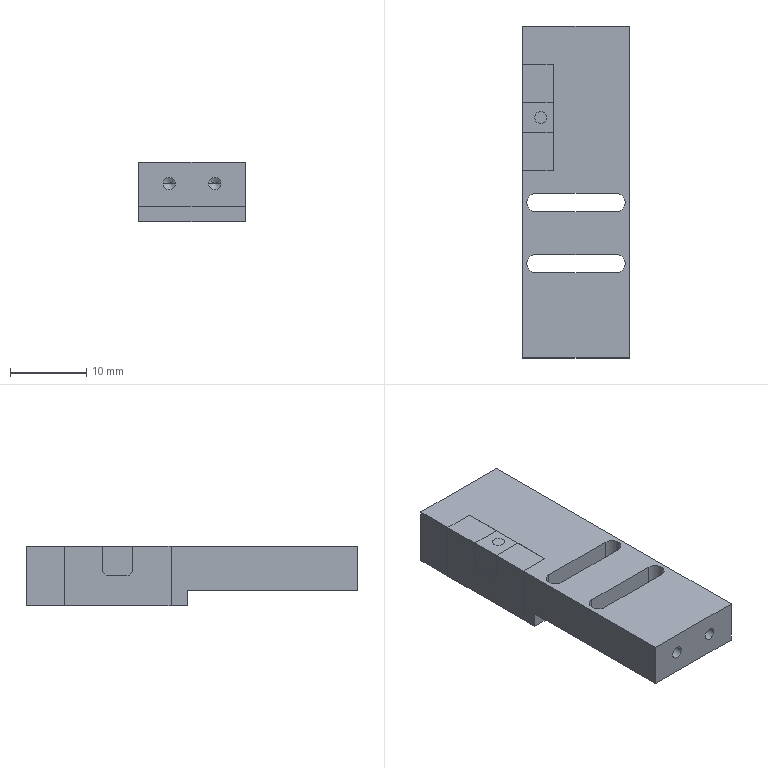NC program | NX | posted with a generic post | part box 14 x 43.5 x 7.8 mm
Whole program:
N10 G17 G21 G94 G90
(FLOOR_WALL , TOOL : D10JING)
N12 T09 M6
N14 G54
N16 G17 G0 G90 X31.75 Y-8.997 B0. C0. S9500 M3
N18 G43 Z30. H9
N20 Z3.
N22 G94 G1 Z0. F1250.
N24 X28.75
N26 X-28.75
N28 Y-4.331
N30 X28.75
N32 Y0.334
N34 X-28.75
N36 Y5.
N38 X28.75
N40 X31.75
N42 Z3.
N44 G0 Z30.
N46 M5
(DRILLING_COPY_1 , TOOL : D6A45)
N48 T07 M6
N50 G54
N52 G17 G0 G90 X-9.75 Y4.6 B0. C0. S5000 M3
N54 G43 Z30. H7
N56 G94 G81 G98 Z-1. F250. R3.
N58 X5.39 Y3.5
N60 G80
N62 G0 X5.39 Y3.5 Z30.
N64 M5
(DRILLING_COPY_COPY_COPY , TOOL : 1.6ZT)
N66 T14 M6
N68 G54
N70 G17 G0 G90 X-9.75 Y4.6 B0. C0. S2000 M3
N72 G43 Z30. H14
N74 G94 G83 G98 Z-9.781 F150. Q2. R3.
N76 X5.39 Y3.5 Z-6.481
N78 G80
N80 G0 X5.39 Y3.5 Z30.
N82 M5
(ZLEVEL_PROFILE , TOOL : D10)
N84 T10 M6
N86 G54
N88 G17 G0 G90 X14.075 Y12.1 B0. C0. S9500 M3
N90 G43 Z30. H10
N92 Z1.5
N94 G94 G1 X22.304 Z1.069 F1000.
N96 X23.648 Y11.766 Z0.996
N98 X24.854 Y11.084 Z0.924
N100 X25.834 Y10.104 Z0.851
N102 X26.516 Y8.898 Z0.778
N104 X26.85 Y7.554 Z0.706
N106 Y-7.554 Z-0.086
N108 X26.516 Y-8.898 Z-0.159
N110 X25.834 Y-10.104 Z-0.231
N112 X24.854 Y-11.084 Z-0.304
N114 X23.648 Y-11.766 Z-0.376
N116 X22.304 Y-12.1 Z-0.449
N118 X21.75 Z-0.478
N120 X-21.75 F2500.
N122 G2 X-26.85 Y-7. R5.1
N124 G1 Y7.
N126 G2 X-21.75 Y12.1 R5.1
N128 G1 X21.75
N130 G2 X26.85 Y7. R5.1
N132 G1 Y-7.
N134 G2 X21.75 Y-12.1 R5.1
N136 G1 X-5.642 Z-0.956
N138 X-21.75
N140 G2 X-26.85 Y-7. R5.1
N142 G1 Y7.
N144 G2 X-21.75 Y12.1 R5.1
N146 G1 X21.75
N148 G2 X26.85 Y7. R5.1
N150 G1 Y-7.
N152 G2 X21.75 Y-12.1 R5.1
N154 G1 X-5.642 Z-1.434
N156 X-21.75
N158 G2 X-26.85 Y-7. R5.1
N160 G1 Y7.
N162 G2 X-21.75 Y12.1 R5.1
N164 G1 X21.75
N166 G2 X26.85 Y7. R5.1
N168 G1 Y-7.
N170 G2 X21.75 Y-12.1 R5.1
N172 G1 X-5.642 Z-1.913
N174 X-21.75
N176 G2 X-26.85 Y-7. R5.1
N178 G1 Y7.
N180 G2 X-21.75 Y12.1 R5.1
N182 G1 X21.75
N184 G2 X26.85 Y7. R5.1
N186 G1 Y-7.
N188 G2 X21.75 Y-12.1 R5.1
N190 G1 X-5.642 Z-2.391
N192 X-21.75
N194 G2 X-26.85 Y-7. R5.1
N196 G1 Y7.
N198 G2 X-21.75 Y12.1 R5.1
N200 G1 X21.75
N202 G2 X26.85 Y7. R5.1
N204 G1 Y-7.
N206 G2 X21.75 Y-12.1 R5.1
N208 G1 X-5.642 Z-2.869
N210 X-21.75
N212 G2 X-26.85 Y-7. R5.1
N214 G1 Y7.
N216 G2 X-21.75 Y12.1 R5.1
N218 G1 X21.75
N220 G2 X26.85 Y7. R5.1
N222 G1 Y-7.
N224 G2 X21.75 Y-12.1 R5.1
N226 G1 X-5.642 Z-3.347
N228 X-21.75
N230 G2 X-26.85 Y-7. R5.1
N232 G1 Y7.
N234 G2 X-21.75 Y12.1 R5.1
N236 G1 X21.75
N238 G2 X26.85 Y7. R5.1
N240 G1 Y-7.
N242 G2 X21.75 Y-12.1 R5.1
N244 G1 X-5.642 Z-3.825
N246 X-21.75
N248 G2 X-26.85 Y-7. R5.1
N250 G1 Y7.
N252 G2 X-21.75 Y12.1 R5.1
N254 G1 X21.75
N256 G2 X26.85 Y7. R5.1
N258 G1 Y-7.
N260 G2 X21.75 Y-12.1 R5.1
N262 G1 X-5.642 Z-4.303
N264 X-21.75
N266 G2 X-26.85 Y-7. R5.1
N268 G1 Y7.
N270 G2 X-21.75 Y12.1 R5.1
N272 G1 X21.75
N274 G2 X26.85 Y7. R5.1
N276 G1 Y-7.
N278 G2 X21.75 Y-12.1 R5.1
N280 G1 X-5.642 Z-4.781
N282 X-21.75
N284 G2 X-26.85 Y-7. R5.1
N286 G1 Y7.
N288 G2 X-21.75 Y12.1 R5.1
N290 G1 X21.75
N292 G2 X26.85 Y7. R5.1
N294 G1 Y-7.
N296 G2 X21.75 Y-12.1 R5.1
N298 G1 X-5.642 Z-5.259
N300 X-21.75
N302 G2 X-26.85 Y-7. R5.1
N304 G1 Y7.
N306 G2 X-21.75 Y12.1 R5.1
N308 G1 X21.75
N310 G2 X26.85 Y7. R5.1
N312 G1 Y-7.
N314 G2 X21.75 Y-12.1 R5.1
N316 G1 X-5.642 Z-5.738
N318 X-21.75
N320 G2 X-26.85 Y-7. R5.1
N322 G1 Y7.
N324 G2 X-21.75 Y12.1 R5.1
N326 G1 X21.75
N328 G2 X26.85 Y7. R5.1
N330 G1 Y-7.
N332 G2 X21.75 Y-12.1 R5.1
N334 G1 X-5.642 Z-6.216
N336 X-21.75
N338 G2 X-26.85 Y-7. R5.1
N340 G1 Y7.
N342 G2 X-21.75 Y12.1 R5.1
N344 G1 X21.75
N346 G2 X26.85 Y7. R5.1
N348 G1 Y-7.
N350 G2 X21.75 Y-12.1 R5.1
N352 G1 X-5.642 Z-6.694
N354 X-21.75
N356 G2 X-26.85 Y-7. R5.1
N358 G1 Y7.
N360 G2 X-21.75 Y12.1 R5.1
N362 G1 X21.75
N364 G2 X26.85 Y7. R5.1
N366 G1 Y-7.
N368 G2 X21.75 Y-12.1 R5.1
N370 G1 X-5.642 Z-7.172
N372 X-21.75
N374 G2 X-26.85 Y-7. R5.1
N376 G1 Y7.
N378 G2 X-21.75 Y12.1 R5.1
N380 G1 X21.75
N382 G2 X26.85 Y7. R5.1
N384 G1 Y-7.
N386 G2 X21.75 Y-12.1 R5.1
N388 G1 X-5.642 Z-7.65
N390 X-21.75
N392 G2 X-26.85 Y-7. R5.1
N394 G1 Y7.
N396 G2 X-21.75 Y12.1 R5.1
N398 G1 X21.75
N400 G2 X26.85 Y7. R5.1
N402 G1 Y-7.
N404 G2 X21.75 Y-12.1 R5.1
N406 G1 X-5.642
N408 Z-6.15
N410 G0 Z30.
N412 M5
(FLOOR_WALL_1 , TOOL : D6)
N414 T06 M6
N416 G54
N418 G17 G0 G90 X12.12 Y12. B0. C0. S9500 M3
N420 G43 Z30. H6
N422 Z0.525
N424 G94 G1 Z-0.475 F1000.
N426 Y7.
N428 X21.75 F2500.
N430 Y-7.
N432 X2.49
N434 Y7.
N436 X12.12
N438 Y4.
N440 X18.75
N442 Y-4.
N444 X5.49
N446 Y4.
N448 X12.12
N450 Y1.
N452 X15.75
N454 Y-1.
N456 X8.49
N458 Y1.
N460 X12.12
N462 Y2.
N464 Z0.525
N466 G0 Y12. Z0.05
N468 G1 Z-0.95 F1000.
N470 Y7.
N472 X21.75 F2500.
N474 Y-7.
N476 X2.49
N478 Y7.
N480 X12.12
N482 Y4.
N484 X18.75
N486 Y-4.
N488 X5.49
N490 Y4.
N492 X12.12
N494 Y1.
N496 X15.75
N498 Y-1.
N500 X8.49
N502 Y1.
N504 X12.12
N506 Y2.
N508 Z0.05
N510 G0 Y12. Z-0.425
N512 G1 Z-1.425 F1000.
N514 Y7.
N516 X21.75 F2500.
N518 Y-7.
N520 X2.49
N522 Y7.
N524 X12.12
N526 Y4.
N528 X18.75
N530 Y-4.
N532 X5.49
N534 Y4.
N536 X12.12
N538 Y1.
N540 X15.75
N542 Y-1.
N544 X8.49
N546 Y1.
N548 X12.12
N550 Y2.
N552 Z-0.425
N554 G0 Y12. Z-0.9
N556 G1 Z-1.9 F1000.
N558 Y7.
N560 X21.75 F2500.
N562 Y-7.
N564 X2.49
N566 Y7.
N568 X12.12
N570 Y4.
N572 X18.75
N574 Y-4.
N576 X5.49
N578 Y4.
N580 X12.12
N582 Y1.
N584 X15.75
N586 Y-1.
N588 X8.49
N590 Y1.
N592 X12.12
N594 Y2.
N596 Z-0.9
N598 G0 Z30.
(FLOOR_WALL_1_COPY , TOOL : D6)
N600 X21.747 Y12.
N602 Z-1.
N604 G1 Z-2. F1000.
N606 Y10.
N608 Y-10. F1200.
N610 X19.025
N612 Y10.
N614 X16.302
N616 Y-10.
N618 X13.58
N620 Y10.
N622 X10.857
N624 Y-10.
N626 X8.135
N628 Y10.
N630 X5.412
N632 Y-10.
N634 X2.69
N636 Y10.
N638 Y12.
N640 Z-1.
N642 G0 X2.39
N644 G1 Z-2. F1000.
N646 Y10.
N648 Y-10. F1200.
N650 Y-12.
N652 Z-1.
N654 G0 Z30.
N656 M5
(ZLEVEL_PROFILE_COPY_COPY_COPY , TOOL : D1.5)
N658 T13 M6
N660 G54
N662 G17 G0 G90 X1.84 Y0.019 B0. C0. S9500 M3
N664 G43 Z30. H13
N666 Z-0.5
N668 G94 G1 Y5.345 Z-0.779 F1000.
N670 X1.754 Y5.531 Z-0.79
N672 X1.597 Y5.661 Z-0.801
N674 X1.398 Y5.71 Z-0.811
N676 X1.211 Y5.674 Z-0.821
N678 X1.035 Y5.543 Z-0.833
N680 X0.94 Y5.345 Z-0.844
N682 Y-5.345 Z-1.405
N684 X1.026 Y-5.531 Z-1.415
N686 X1.183 Y-5.661 Z-1.426
N688 X1.382 Y-5.71 Z-1.437
N690 X1.569 Y-5.674 Z-1.447
N692 X1.745 Y-5.543 Z-1.458
N694 X1.84 Y-5.345 Z-1.47
N696 Y5.345 Z-2.03
N698 X1.754 Y5.531 Z-2.041
N700 X1.597 Y5.661 Z-2.051
N702 X1.398 Y5.71 Z-2.062
N704 X1.211 Y5.674 Z-2.072
N706 X1.035 Y5.543 Z-2.084
N708 X0.94 Y5.345 Z-2.095
N710 Y5.25 Z-2.1
N712 Y-5.25
N714 G3 X1.39 Y-5.7 R0.45
N716 X1.84 Y-5.25 R0.45
N718 G1 Y5.25
N720 G3 X1.39 Y5.7 R0.45
N722 X0.94 Y5.25 R0.45
N724 G1 Y-0.479 Z-2.2
N726 Y-5.25
N728 G3 X1.39 Y-5.7 R0.45
N730 X1.84 Y-5.25 R0.45
N732 G1 Y5.25
N734 G3 X1.39 Y5.7 R0.45
N736 X0.94 Y5.25 R0.45
N738 G1 Y-0.479 Z-2.3
N740 Y-5.25
N742 G3 X1.39 Y-5.7 R0.45
N744 X1.84 Y-5.25 R0.45
N746 G1 Y5.25
N748 G3 X1.39 Y5.7 R0.45
N750 X0.94 Y5.25 R0.45
N752 G1 Y-0.479 Z-2.4
N754 Y-5.25
N756 G3 X1.39 Y-5.7 R0.45
N758 X1.84 Y-5.25 R0.45
N760 G1 Y5.25
N762 G3 X1.39 Y5.7 R0.45
N764 X0.94 Y5.25 R0.45
N766 G1 Y-0.479 Z-2.5
N768 Y-5.25
N770 G3 X1.39 Y-5.7 R0.45
N772 X1.84 Y-5.25 R0.45
N774 G1 Y5.25
N776 G3 X1.39 Y5.7 R0.45
N778 X0.94 Y5.25 R0.45
N780 G1 Y-0.479 Z-2.6
N782 Y-5.25
N784 G3 X1.39 Y-5.7 R0.45
N786 X1.84 Y-5.25 R0.45
N788 G1 Y5.25
N790 G3 X1.39 Y5.7 R0.45
N792 X0.94 Y5.25 R0.45
N794 G1 Y-0.479 Z-2.7
N796 Y-5.25
N798 G3 X1.39 Y-5.7 R0.45
N800 X1.84 Y-5.25 R0.45
N802 G1 Y5.25
N804 G3 X1.39 Y5.7 R0.45
N806 X0.94 Y5.25 R0.45
N808 G1 Y-0.479 Z-2.8
N810 Y-5.25
N812 G3 X1.39 Y-5.7 R0.45
N814 X1.84 Y-5.25 R0.45
N816 G1 Y5.25
N818 G3 X1.39 Y5.7 R0.45
N820 X0.94 Y5.25 R0.45
N822 G1 Y-0.479 Z-2.9
N824 Y-5.25
N826 G3 X1.39 Y-5.7 R0.45
N828 X1.84 Y-5.25 R0.45
N830 G1 Y5.25
N832 G3 X1.39 Y5.7 R0.45
N834 X0.94 Y5.25 R0.45
N836 G1 Y-0.479 Z-3.
N838 Y-5.25
N840 G3 X1.39 Y-5.7 R0.45
N842 X1.84 Y-5.25 R0.45
N844 G1 Y5.25
N846 G3 X1.39 Y5.7 R0.45
N848 X0.94 Y5.25 R0.45
N850 G1 Y-0.479 Z-3.1
N852 Y-5.25
N854 G3 X1.39 Y-5.7 R0.45
N856 X1.84 Y-5.25 R0.45
N858 G1 Y5.25
N860 G3 X1.39 Y5.7 R0.45
N862 X0.94 Y5.25 R0.45
N864 G1 Y-0.479 Z-3.2
N866 Y-5.25
N868 G3 X1.39 Y-5.7 R0.45
N870 X1.84 Y-5.25 R0.45
N872 G1 Y5.25
N874 G3 X1.39 Y5.7 R0.45
N876 X0.94 Y5.25 R0.45
N878 G1 Y-0.479 Z-3.3
N880 Y-5.25
N882 G3 X1.39 Y-5.7 R0.45
N884 X1.84 Y-5.25 R0.45
N886 G1 Y5.25
N888 G3 X1.39 Y5.7 R0.45
N890 X0.94 Y5.25 R0.45
N892 G1 Y-0.479 Z-3.4
N894 Y-5.25
N896 G3 X1.39 Y-5.7 R0.45
N898 X1.84 Y-5.25 R0.45
N900 G1 Y5.25
N902 G3 X1.39 Y5.7 R0.45
N904 X0.94 Y5.25 R0.45
N906 G1 Y-0.479 Z-3.5
N908 Y-5.25
N910 G3 X1.39 Y-5.7 R0.45
N912 X1.84 Y-5.25 R0.45
N914 G1 Y5.25
N916 G3 X1.39 Y5.7 R0.45
N918 X0.94 Y5.25 R0.45
N920 G1 Y-0.479 Z-3.6
N922 Y-5.25
N924 G3 X1.39 Y-5.7 R0.45
N926 X1.84 Y-5.25 R0.45
N928 G1 Y5.25
N930 G3 X1.39 Y5.7 R0.45
N932 X0.94 Y5.25 R0.45
N934 G1 Y-0.479 Z-3.7
N936 Y-5.25
N938 G3 X1.39 Y-5.7 R0.45
N940 X1.84 Y-5.25 R0.45
N942 G1 Y5.25
N944 G3 X1.39 Y5.7 R0.45
N946 X0.94 Y5.25 R0.45
N948 G1 Y-0.479 Z-3.8
N950 Y-5.25
N952 G3 X1.39 Y-5.7 R0.45
N954 X1.84 Y-5.25 R0.45
N956 G1 Y5.25
N958 G3 X1.39 Y5.7 R0.45
N960 X0.94 Y5.25 R0.45
N962 G1 Y-0.479 Z-3.9
N964 Y-5.25
N966 G3 X1.39 Y-5.7 R0.45
N968 X1.84 Y-5.25 R0.45
N970 G1 Y5.25
N972 G3 X1.39 Y5.7 R0.45
N974 X0.94 Y5.25 R0.45
N976 G1 Y-0.479 Z-4.
N978 Y-5.25
N980 G3 X1.39 Y-5.7 R0.45
N982 X1.84 Y-5.25 R0.45
N984 G1 Y5.25
N986 G3 X1.39 Y5.7 R0.45
N988 X0.94 Y5.25 R0.45
N990 G1 Y-0.479 Z-4.1
N992 Y-5.25
N994 G3 X1.39 Y-5.7 R0.45
N996 X1.84 Y-5.25 R0.45
N998 G1 Y5.25
N1000 G3 X1.39 Y5.7 R0.45
N1002 X0.94 Y5.25 R0.45
N1004 G1 Y-0.479 Z-4.2
N1006 Y-5.25
N1008 G3 X1.39 Y-5.7 R0.45
N1010 X1.84 Y-5.25 R0.45
N1012 G1 Y5.25
N1014 G3 X1.39 Y5.7 R0.45
N1016 X0.94 Y5.25 R0.45
N1018 G1 Y-0.479 Z-4.3
N1020 Y-5.25
N1022 G3 X1.39 Y-5.7 R0.45
N1024 X1.84 Y-5.25 R0.45
N1026 G1 Y5.25
N1028 G3 X1.39 Y5.7 R0.45
N1030 X0.94 Y5.25 R0.45
N1032 G1 Y-0.479 Z-4.4
N1034 Y-5.25
N1036 G3 X1.39 Y-5.7 R0.45
N1038 X1.84 Y-5.25 R0.45
N1040 G1 Y5.25
N1042 G3 X1.39 Y5.7 R0.45
N1044 X0.94 Y5.25 R0.45
N1046 G1 Y-0.479 Z-4.5
N1048 Y-5.25
N1050 G3 X1.39 Y-5.7 R0.45
N1052 X1.84 Y-5.25 R0.45
N1054 G1 Y5.25
N1056 G3 X1.39 Y5.7 R0.45
N1058 X0.94 Y5.25 R0.45
N1060 G1 Y-0.479 Z-4.6
N1062 Y-5.25
N1064 G3 X1.39 Y-5.7 R0.45
N1066 X1.84 Y-5.25 R0.45
N1068 G1 Y5.25
N1070 G3 X1.39 Y5.7 R0.45
N1072 X0.94 Y5.25 R0.45
N1074 G1 Y-0.479 Z-4.7
N1076 Y-5.25
N1078 G3 X1.39 Y-5.7 R0.45
N1080 X1.84 Y-5.25 R0.45
N1082 G1 Y5.25
N1084 G3 X1.39 Y5.7 R0.45
N1086 X0.94 Y5.25 R0.45
N1088 G1 Y-0.479 Z-4.8
N1090 Y-5.25
N1092 G3 X1.39 Y-5.7 R0.45
N1094 X1.84 Y-5.25 R0.45
N1096 G1 Y5.25
N1098 G3 X1.39 Y5.7 R0.45
N1100 X0.94 Y5.25 R0.45
N1102 G1 Y-0.479 Z-4.9
N1104 Y-5.25
N1106 G3 X1.39 Y-5.7 R0.45
N1108 X1.84 Y-5.25 R0.45
N1110 G1 Y5.25
N1112 G3 X1.39 Y5.7 R0.45
N1114 X0.94 Y5.25 R0.45
N1116 G1 Y-0.479 Z-5.
N1118 Y-5.25
N1120 G3 X1.39 Y-5.7 R0.45
N1122 X1.84 Y-5.25 R0.45
N1124 G1 Y5.25
N1126 G3 X1.39 Y5.7 R0.45
N1128 X0.94 Y5.25 R0.45
N1130 G1 Y-0.479 Z-5.1
N1132 Y-5.25
N1134 G3 X1.39 Y-5.7 R0.45
N1136 X1.84 Y-5.25 R0.45
N1138 G1 Y5.25
N1140 G3 X1.39 Y5.7 R0.45
N1142 X0.94 Y5.25 R0.45
N1144 G1 Y-0.479 Z-5.2
N1146 Y-5.25
N1148 G3 X1.39 Y-5.7 R0.45
N1150 X1.84 Y-5.25 R0.45
N1152 G1 Y5.25
N1154 G3 X1.39 Y5.7 R0.45
N1156 X0.94 Y5.25 R0.45
N1158 G1 Y-0.479 Z-5.3
N1160 Y-5.25
N1162 G3 X1.39 Y-5.7 R0.45
N1164 X1.84 Y-5.25 R0.45
N1166 G1 Y5.25
N1168 G3 X1.39 Y5.7 R0.45
N1170 X0.94 Y5.25 R0.45
N1172 G1 Y-0.479 Z-5.4
N1174 Y-5.25
N1176 G3 X1.39 Y-5.7 R0.45
N1178 X1.84 Y-5.25 R0.45
N1180 G1 Y5.25
N1182 G3 X1.39 Y5.7 R0.45
N1184 X0.94 Y5.25 R0.45
N1186 G1 Y-0.479 Z-5.5
N1188 Y-5.25
N1190 G3 X1.39 Y-5.7 R0.45
N1192 X1.84 Y-5.25 R0.45
N1194 G1 Y5.25
N1196 G3 X1.39 Y5.7 R0.45
N1198 X0.94 Y5.25 R0.45
N1200 G1 Y-0.479 Z-5.6
N1202 Y-5.25
N1204 G3 X1.39 Y-5.7 R0.45
N1206 X1.84 Y-5.25 R0.45
N1208 G1 Y5.25
N1210 G3 X1.39 Y5.7 R0.45
N1212 X0.94 Y5.25 R0.45
N1214 G1 Y-0.479 Z-5.7
N1216 Y-5.25
N1218 G3 X1.39 Y-5.7 R0.45
N1220 X1.84 Y-5.25 R0.45
N1222 G1 Y5.25
N1224 G3 X1.39 Y5.7 R0.45
N1226 X0.94 Y5.25 R0.45
N1228 G1 Y-0.479 Z-5.8
N1230 Y-5.25
N1232 G3 X1.39 Y-5.7 R0.45
N1234 X1.84 Y-5.25 R0.45
N1236 G1 Y5.25
N1238 G3 X1.39 Y5.7 R0.45
N1240 X0.94 Y5.25 R0.45
N1242 G1 Y-0.479 Z-5.9
N1244 Y-5.25
N1246 G3 X1.39 Y-5.7 R0.45
N1248 X1.84 Y-5.25 R0.45
N1250 G1 Y5.25
N1252 G3 X1.39 Y5.7 R0.45
N1254 X0.94 Y5.25 R0.45
N1256 G1 Y-0.479 Z-6.
N1258 Y-5.25
N1260 G3 X1.39 Y-5.7 R0.45
N1262 X1.84 Y-5.25 R0.45
N1264 G1 Y5.25
N1266 G3 X1.39 Y5.7 R0.45
N1268 X0.94 Y5.25 R0.45
N1270 G1 Y-0.479 Z-6.1
N1272 Y-5.25
N1274 G3 X1.39 Y-5.7 R0.45
N1276 X1.84 Y-5.25 R0.45
N1278 G1 Y5.25
N1280 G3 X1.39 Y5.7 R0.45
N1282 X0.94 Y5.25 R0.45
N1284 G1 Y-0.479 Z-6.2
N1286 Y-5.25
N1288 G3 X1.39 Y-5.7 R0.45
N1290 X1.84 Y-5.25 R0.45
N1292 G1 Y5.25
N1294 G3 X1.39 Y5.7 R0.45
N1296 X0.94 Y5.25 R0.45
N1298 G1 Y-0.479 Z-6.3
N1300 Y-5.25
N1302 G3 X1.39 Y-5.7 R0.45
N1304 X1.84 Y-5.25 R0.45
N1306 G1 Y5.25
N1308 G3 X1.39 Y5.7 R0.45
N1310 X0.94 Y5.25 R0.45
N1312 G1 Y-0.479 Z-6.4
N1314 Y-5.25
N1316 G3 X1.39 Y-5.7 R0.45
N1318 X1.84 Y-5.25 R0.45
N1320 G1 Y5.25
N1322 G3 X1.39 Y5.7 R0.45
N1324 X0.94 Y5.25 R0.45
N1326 G1 Y-0.479 Z-6.5
N1328 Y-5.25
N1330 G3 X1.39 Y-5.7 R0.45
N1332 X1.84 Y-5.25 R0.45
N1334 G1 Y5.25
N1336 G3 X1.39 Y5.7 R0.45
N1338 X0.94 Y5.25 R0.45
N1340 G1 Y-0.479 Z-6.6
N1342 Y-5.25
N1344 G3 X1.39 Y-5.7 R0.45
N1346 X1.84 Y-5.25 R0.45
N1348 G1 Y5.25
N1350 G3 X1.39 Y5.7 R0.45
N1352 X0.94 Y5.25 R0.45
N1354 G1 Y-0.479 Z-6.7
N1356 Y-5.25
N1358 G3 X1.39 Y-5.7 R0.45
N1360 X1.84 Y-5.25 R0.45
N1362 G1 Y5.25
N1364 G3 X1.39 Y5.7 R0.45
N1366 X0.94 Y5.25 R0.45
N1368 G1 Y-0.479 Z-6.8
N1370 Y-5.25
N1372 G3 X1.39 Y-5.7 R0.45
N1374 X1.84 Y-5.25 R0.45
N1376 G1 Y5.25
N1378 G3 X1.39 Y5.7 R0.45
N1380 X0.94 Y5.25 R0.45
N1382 G1 Y-0.479 Z-6.9
N1384 Y-5.25
N1386 G3 X1.39 Y-5.7 R0.45
N1388 X1.84 Y-5.25 R0.45
N1390 G1 Y5.25
N1392 G3 X1.39 Y5.7 R0.45
N1394 X0.94 Y5.25 R0.45
N1396 G1 Y-0.479 Z-7.
N1398 Y-5.25
N1400 G3 X1.39 Y-5.7 R0.45
N1402 X1.84 Y-5.25 R0.45
N1404 G1 Y5.25
N1406 G3 X1.39 Y5.7 R0.45
N1408 X0.94 Y5.25 R0.45
N1410 G1 Y-0.479 Z-7.1
N1412 Y-5.25
N1414 G3 X1.39 Y-5.7 R0.45
N1416 X1.84 Y-5.25 R0.45
N1418 G1 Y5.25
N1420 G3 X1.39 Y5.7 R0.45
N1422 X0.94 Y5.25 R0.45
N1424 G1 Y-0.479 Z-7.2
N1426 Y-5.25
N1428 G3 X1.39 Y-5.7 R0.45
N1430 X1.84 Y-5.25 R0.45
N1432 G1 Y5.25
N1434 G3 X1.39 Y5.7 R0.45
N1436 X0.94 Y5.25 R0.45
N1438 G1 Y-0.479 Z-7.3
N1440 Y-5.25
N1442 G3 X1.39 Y-5.7 R0.45
N1444 X1.84 Y-5.25 R0.45
N1446 G1 Y5.25
N1448 G3 X1.39 Y5.7 R0.45
N1450 X0.94 Y5.25 R0.45
N1452 G1 Y-0.479 Z-7.4
N1454 Y-5.25
N1456 G3 X1.39 Y-5.7 R0.45
N1458 X1.84 Y-5.25 R0.45
N1460 G1 Y5.25
N1462 G3 X1.39 Y5.7 R0.45
N1464 X0.94 Y5.25 R0.45
N1466 G1 Y-0.479 Z-7.5
N1468 Y-5.25
N1470 G3 X1.39 Y-5.7 R0.45
N1472 X1.84 Y-5.25 R0.45
N1474 G1 Y5.25
N1476 G3 X1.39 Y5.7 R0.45
N1478 X0.94 Y5.25 R0.45
N1480 G1 Y-0.479 Z-7.6
N1482 Y-5.25
N1484 G3 X1.39 Y-5.7 R0.45
N1486 X1.84 Y-5.25 R0.45
N1488 G1 Y5.25
N1490 G3 X1.39 Y5.7 R0.45
N1492 X0.94 Y5.25 R0.45
N1494 G1 Y-0.479 Z-7.7
N1496 Y-5.25
N1498 G3 X1.39 Y-5.7 R0.45
N1500 X1.84 Y-5.25 R0.45
N1502 G1 Y5.25
N1504 G3 X1.39 Y5.7 R0.45
N1506 X0.94 Y5.25 R0.45
N1508 G1 Y-0.479 Z-7.8
N1510 Y-5.25
N1512 G3 X1.39 Y-5.7 R0.45
N1514 X1.84 Y-5.25 R0.45
N1516 G1 Y5.25
N1518 G3 X1.39 Y5.7 R0.45
N1520 X0.94 Y5.25 R0.45
N1522 G1 Y-0.479
N1524 Z-6.3
N1526 G0 Z30.
N1528 X9.84 Y0.019
N1530 Z-0.5
N1532 G1 Y5.345 Z-0.779
N1534 X9.754 Y5.531 Z-0.79
N1536 X9.597 Y5.661 Z-0.801
N1538 X9.398 Y5.71 Z-0.811
N1540 X9.211 Y5.674 Z-0.821
N1542 X9.035 Y5.543 Z-0.833
N1544 X8.94 Y5.345 Z-0.844
N1546 Y-5.345 Z-1.405
N1548 X9.026 Y-5.531 Z-1.415
N1550 X9.183 Y-5.661 Z-1.426
N1552 X9.382 Y-5.71 Z-1.437
N1554 X9.569 Y-5.674 Z-1.447
N1556 X9.745 Y-5.543 Z-1.458
N1558 X9.84 Y-5.345 Z-1.47
N1560 Y5.345 Z-2.03
N1562 X9.754 Y5.531 Z-2.041
N1564 X9.597 Y5.661 Z-2.051
N1566 X9.398 Y5.71 Z-2.062
N1568 X9.211 Y5.674 Z-2.072
N1570 X9.035 Y5.543 Z-2.084
N1572 X8.94 Y5.345 Z-2.095
N1574 Y5.25 Z-2.1
N1576 Y-5.25
N1578 G3 X9.39 Y-5.7 R0.45
N1580 X9.84 Y-5.25 R0.45
N1582 G1 Y5.25
N1584 G3 X9.39 Y5.7 R0.45
N1586 X8.94 Y5.25 R0.45
N1588 G1 Y-0.479 Z-2.2
N1590 Y-5.25
N1592 G3 X9.39 Y-5.7 R0.45
N1594 X9.84 Y-5.25 R0.45
N1596 G1 Y5.25
N1598 G3 X9.39 Y5.7 R0.45
N1600 X8.94 Y5.25 R0.45
N1602 G1 Y-0.479 Z-2.3
N1604 Y-5.25
N1606 G3 X9.39 Y-5.7 R0.45
N1608 X9.84 Y-5.25 R0.45
N1610 G1 Y5.25
N1612 G3 X9.39 Y5.7 R0.45
N1614 X8.94 Y5.25 R0.45
N1616 G1 Y-0.479 Z-2.4
N1618 Y-5.25
N1620 G3 X9.39 Y-5.7 R0.45
N1622 X9.84 Y-5.25 R0.45
N1624 G1 Y5.25
N1626 G3 X9.39 Y5.7 R0.45
N1628 X8.94 Y5.25 R0.45
N1630 G1 Y-0.479 Z-2.5
N1632 Y-5.25
N1634 G3 X9.39 Y-5.7 R0.45
N1636 X9.84 Y-5.25 R0.45
N1638 G1 Y5.25
N1640 G3 X9.39 Y5.7 R0.45
N1642 X8.94 Y5.25 R0.45
N1644 G1 Y-0.479 Z-2.6
N1646 Y-5.25
N1648 G3 X9.39 Y-5.7 R0.45
N1650 X9.84 Y-5.25 R0.45
N1652 G1 Y5.25
N1654 G3 X9.39 Y5.7 R0.45
N1656 X8.94 Y5.25 R0.45
N1658 G1 Y-0.479 Z-2.7
N1660 Y-5.25
N1662 G3 X9.39 Y-5.7 R0.45
N1664 X9.84 Y-5.25 R0.45
N1666 G1 Y5.25
N1668 G3 X9.39 Y5.7 R0.45
N1670 X8.94 Y5.25 R0.45
N1672 G1 Y-0.479 Z-2.8
N1674 Y-5.25
N1676 G3 X9.39 Y-5.7 R0.45
N1678 X9.84 Y-5.25 R0.45
N1680 G1 Y5.25
N1682 G3 X9.39 Y5.7 R0.45
N1684 X8.94 Y5.25 R0.45
N1686 G1 Y-0.479 Z-2.9
N1688 Y-5.25
N1690 G3 X9.39 Y-5.7 R0.45
N1692 X9.84 Y-5.25 R0.45
N1694 G1 Y5.25
N1696 G3 X9.39 Y5.7 R0.45
N1698 X8.94 Y5.25 R0.45
N1700 G1 Y-0.479 Z-3.
N1702 Y-5.25
N1704 G3 X9.39 Y-5.7 R0.45
N1706 X9.84 Y-5.25 R0.45
N1708 G1 Y5.25
N1710 G3 X9.39 Y5.7 R0.45
N1712 X8.94 Y5.25 R0.45
N1714 G1 Y-0.479 Z-3.1
N1716 Y-5.25
N1718 G3 X9.39 Y-5.7 R0.45
N1720 X9.84 Y-5.25 R0.45
N1722 G1 Y5.25
N1724 G3 X9.39 Y5.7 R0.45
N1726 X8.94 Y5.25 R0.45
N1728 G1 Y-0.479 Z-3.2
N1730 Y-5.25
N1732 G3 X9.39 Y-5.7 R0.45
N1734 X9.84 Y-5.25 R0.45
N1736 G1 Y5.25
N1738 G3 X9.39 Y5.7 R0.45
N1740 X8.94 Y5.25 R0.45
N1742 G1 Y-0.479 Z-3.3
N1744 Y-5.25
N1746 G3 X9.39 Y-5.7 R0.45
N1748 X9.84 Y-5.25 R0.45
N1750 G1 Y5.25
N1752 G3 X9.39 Y5.7 R0.45
N1754 X8.94 Y5.25 R0.45
N1756 G1 Y-0.479 Z-3.4
N1758 Y-5.25
N1760 G3 X9.39 Y-5.7 R0.45
N1762 X9.84 Y-5.25 R0.45
N1764 G1 Y5.25
N1766 G3 X9.39 Y5.7 R0.45
N1768 X8.94 Y5.25 R0.45
N1770 G1 Y-0.479 Z-3.5
N1772 Y-5.25
N1774 G3 X9.39 Y-5.7 R0.45
N1776 X9.84 Y-5.25 R0.45
N1778 G1 Y5.25
N1780 G3 X9.39 Y5.7 R0.45
N1782 X8.94 Y5.25 R0.45
N1784 G1 Y-0.479 Z-3.6
N1786 Y-5.25
N1788 G3 X9.39 Y-5.7 R0.45
N1790 X9.84 Y-5.25 R0.45
N1792 G1 Y5.25
N1794 G3 X9.39 Y5.7 R0.45
N1796 X8.94 Y5.25 R0.45
N1798 G1 Y-0.479 Z-3.7
N1800 Y-5.25
N1802 G3 X9.39 Y-5.7 R0.45
N1804 X9.84 Y-5.25 R0.45
N1806 G1 Y5.25
N1808 G3 X9.39 Y5.7 R0.45
N1810 X8.94 Y5.25 R0.45
N1812 G1 Y-0.479 Z-3.8
N1814 Y-5.25
N1816 G3 X9.39 Y-5.7 R0.45
N1818 X9.84 Y-5.25 R0.45
N1820 G1 Y5.25
N1822 G3 X9.39 Y5.7 R0.45
N1824 X8.94 Y5.25 R0.45
N1826 G1 Y-0.479 Z-3.9
N1828 Y-5.25
N1830 G3 X9.39 Y-5.7 R0.45
N1832 X9.84 Y-5.25 R0.45
N1834 G1 Y5.25
N1836 G3 X9.39 Y5.7 R0.45
N1838 X8.94 Y5.25 R0.45
N1840 G1 Y-0.479 Z-4.
N1842 Y-5.25
N1844 G3 X9.39 Y-5.7 R0.45
N1846 X9.84 Y-5.25 R0.45
N1848 G1 Y5.25
N1850 G3 X9.39 Y5.7 R0.45
N1852 X8.94 Y5.25 R0.45
N1854 G1 Y-0.479 Z-4.1
N1856 Y-5.25
N1858 G3 X9.39 Y-5.7 R0.45
N1860 X9.84 Y-5.25 R0.45
N1862 G1 Y5.25
N1864 G3 X9.39 Y5.7 R0.45
N1866 X8.94 Y5.25 R0.45
N1868 G1 Y-0.479 Z-4.2
N1870 Y-5.25
N1872 G3 X9.39 Y-5.7 R0.45
N1874 X9.84 Y-5.25 R0.45
N1876 G1 Y5.25
N1878 G3 X9.39 Y5.7 R0.45
N1880 X8.94 Y5.25 R0.45
N1882 G1 Y-0.479 Z-4.3
N1884 Y-5.25
N1886 G3 X9.39 Y-5.7 R0.45
N1888 X9.84 Y-5.25 R0.45
N1890 G1 Y5.25
N1892 G3 X9.39 Y5.7 R0.45
N1894 X8.94 Y5.25 R0.45
N1896 G1 Y-0.479 Z-4.4
N1898 Y-5.25
N1900 G3 X9.39 Y-5.7 R0.45
N1902 X9.84 Y-5.25 R0.45
N1904 G1 Y5.25
N1906 G3 X9.39 Y5.7 R0.45
N1908 X8.94 Y5.25 R0.45
N1910 G1 Y-0.479 Z-4.5
N1912 Y-5.25
N1914 G3 X9.39 Y-5.7 R0.45
N1916 X9.84 Y-5.25 R0.45
N1918 G1 Y5.25
N1920 G3 X9.39 Y5.7 R0.45
N1922 X8.94 Y5.25 R0.45
N1924 G1 Y-0.479 Z-4.6
N1926 Y-5.25
N1928 G3 X9.39 Y-5.7 R0.45
N1930 X9.84 Y-5.25 R0.45
N1932 G1 Y5.25
N1934 G3 X9.39 Y5.7 R0.45
N1936 X8.94 Y5.25 R0.45
N1938 G1 Y-0.479 Z-4.7
N1940 Y-5.25
N1942 G3 X9.39 Y-5.7 R0.45
N1944 X9.84 Y-5.25 R0.45
N1946 G1 Y5.25
N1948 G3 X9.39 Y5.7 R0.45
N1950 X8.94 Y5.25 R0.45
N1952 G1 Y-0.479 Z-4.8
N1954 Y-5.25
N1956 G3 X9.39 Y-5.7 R0.45
N1958 X9.84 Y-5.25 R0.45
N1960 G1 Y5.25
N1962 G3 X9.39 Y5.7 R0.45
N1964 X8.94 Y5.25 R0.45
N1966 G1 Y-0.479 Z-4.9
N1968 Y-5.25
N1970 G3 X9.39 Y-5.7 R0.45
N1972 X9.84 Y-5.25 R0.45
N1974 G1 Y5.25
N1976 G3 X9.39 Y5.7 R0.45
N1978 X8.94 Y5.25 R0.45
N1980 G1 Y-0.479 Z-5.
N1982 Y-5.25
N1984 G3 X9.39 Y-5.7 R0.45
N1986 X9.84 Y-5.25 R0.45
N1988 G1 Y5.25
N1990 G3 X9.39 Y5.7 R0.45
N1992 X8.94 Y5.25 R0.45
N1994 G1 Y-0.479 Z-5.1
N1996 Y-5.25
N1998 G3 X9.39 Y-5.7 R0.45
N2000 X9.84 Y-5.25 R0.45
N2002 G1 Y5.25
N2004 G3 X9.39 Y5.7 R0.45
N2006 X8.94 Y5.25 R0.45
N2008 G1 Y-0.479 Z-5.2
N2010 Y-5.25
N2012 G3 X9.39 Y-5.7 R0.45
N2014 X9.84 Y-5.25 R0.45
N2016 G1 Y5.25
N2018 G3 X9.39 Y5.7 R0.45
N2020 X8.94 Y5.25 R0.45
N2022 G1 Y-0.479 Z-5.3
N2024 Y-5.25
N2026 G3 X9.39 Y-5.7 R0.45
N2028 X9.84 Y-5.25 R0.45
N2030 G1 Y5.25
N2032 G3 X9.39 Y5.7 R0.45
N2034 X8.94 Y5.25 R0.45
N2036 G1 Y-0.479 Z-5.4
N2038 Y-5.25
N2040 G3 X9.39 Y-5.7 R0.45
N2042 X9.84 Y-5.25 R0.45
N2044 G1 Y5.25
N2046 G3 X9.39 Y5.7 R0.45
N2048 X8.94 Y5.25 R0.45
N2050 G1 Y-0.479 Z-5.5
N2052 Y-5.25
N2054 G3 X9.39 Y-5.7 R0.45
N2056 X9.84 Y-5.25 R0.45
N2058 G1 Y5.25
N2060 G3 X9.39 Y5.7 R0.45
N2062 X8.94 Y5.25 R0.45
N2064 G1 Y-0.479 Z-5.6
N2066 Y-5.25
N2068 G3 X9.39 Y-5.7 R0.45
N2070 X9.84 Y-5.25 R0.45
N2072 G1 Y5.25
N2074 G3 X9.39 Y5.7 R0.45
N2076 X8.94 Y5.25 R0.45
N2078 G1 Y-0.479 Z-5.7
N2080 Y-5.25
N2082 G3 X9.39 Y-5.7 R0.45
N2084 X9.84 Y-5.25 R0.45
N2086 G1 Y5.25
N2088 G3 X9.39 Y5.7 R0.45
N2090 X8.94 Y5.25 R0.45
N2092 G1 Y-0.479 Z-5.8
N2094 Y-5.25
N2096 G3 X9.39 Y-5.7 R0.45
N2098 X9.84 Y-5.25 R0.45
N2100 G1 Y5.25
N2102 G3 X9.39 Y5.7 R0.45
N2104 X8.94 Y5.25 R0.45
N2106 G1 Y-0.479 Z-5.9
N2108 Y-5.25
N2110 G3 X9.39 Y-5.7 R0.45
N2112 X9.84 Y-5.25 R0.45
N2114 G1 Y5.25
N2116 G3 X9.39 Y5.7 R0.45
N2118 X8.94 Y5.25 R0.45
N2120 G1 Y-0.479 Z-6.
N2122 Y-5.25
N2124 G3 X9.39 Y-5.7 R0.45
N2126 X9.84 Y-5.25 R0.45
N2128 G1 Y5.25
N2130 G3 X9.39 Y5.7 R0.45
N2132 X8.94 Y5.25 R0.45
N2134 G1 Y-0.479 Z-6.1
N2136 Y-5.25
N2138 G3 X9.39 Y-5.7 R0.45
N2140 X9.84 Y-5.25 R0.45
N2142 G1 Y5.25
N2144 G3 X9.39 Y5.7 R0.45
N2146 X8.94 Y5.25 R0.45
N2148 G1 Y-0.479 Z-6.2
N2150 Y-5.25
N2152 G3 X9.39 Y-5.7 R0.45
N2154 X9.84 Y-5.25 R0.45
N2156 G1 Y5.25
N2158 G3 X9.39 Y5.7 R0.45
N2160 X8.94 Y5.25 R0.45
N2162 G1 Y-0.479 Z-6.3
N2164 Y-5.25
N2166 G3 X9.39 Y-5.7 R0.45
N2168 X9.84 Y-5.25 R0.45
N2170 G1 Y5.25
N2172 G3 X9.39 Y5.7 R0.45
N2174 X8.94 Y5.25 R0.45
N2176 G1 Y-0.479 Z-6.4
N2178 Y-5.25
N2180 G3 X9.39 Y-5.7 R0.45
N2182 X9.84 Y-5.25 R0.45
N2184 G1 Y5.25
N2186 G3 X9.39 Y5.7 R0.45
N2188 X8.94 Y5.25 R0.45
N2190 G1 Y-0.479 Z-6.5
N2192 Y-5.25
N2194 G3 X9.39 Y-5.7 R0.45
N2196 X9.84 Y-5.25 R0.45
N2198 G1 Y5.25
N2200 G3 X9.39 Y5.7 R0.45
N2202 X8.94 Y5.25 R0.45
N2204 G1 Y-0.479 Z-6.6
N2206 Y-5.25
N2208 G3 X9.39 Y-5.7 R0.45
N2210 X9.84 Y-5.25 R0.45
N2212 G1 Y5.25
N2214 G3 X9.39 Y5.7 R0.45
N2216 X8.94 Y5.25 R0.45
N2218 G1 Y-0.479 Z-6.7
N2220 Y-5.25
N2222 G3 X9.39 Y-5.7 R0.45
N2224 X9.84 Y-5.25 R0.45
N2226 G1 Y5.25
N2228 G3 X9.39 Y5.7 R0.45
N2230 X8.94 Y5.25 R0.45
N2232 G1 Y-0.479 Z-6.8
N2234 Y-5.25
N2236 G3 X9.39 Y-5.7 R0.45
N2238 X9.84 Y-5.25 R0.45
N2240 G1 Y5.25
N2242 G3 X9.39 Y5.7 R0.45
N2244 X8.94 Y5.25 R0.45
N2246 G1 Y-0.479 Z-6.9
N2248 Y-5.25
N2250 G3 X9.39 Y-5.7 R0.45
N2252 X9.84 Y-5.25 R0.45
N2254 G1 Y5.25
N2256 G3 X9.39 Y5.7 R0.45
N2258 X8.94 Y5.25 R0.45
N2260 G1 Y-0.479 Z-7.
N2262 Y-5.25
N2264 G3 X9.39 Y-5.7 R0.45
N2266 X9.84 Y-5.25 R0.45
N2268 G1 Y5.25
N2270 G3 X9.39 Y5.7 R0.45
N2272 X8.94 Y5.25 R0.45
N2274 G1 Y-0.479 Z-7.1
N2276 Y-5.25
N2278 G3 X9.39 Y-5.7 R0.45
N2280 X9.84 Y-5.25 R0.45
N2282 G1 Y5.25
N2284 G3 X9.39 Y5.7 R0.45
N2286 X8.94 Y5.25 R0.45
N2288 G1 Y-0.479 Z-7.2
N2290 Y-5.25
N2292 G3 X9.39 Y-5.7 R0.45
N2294 X9.84 Y-5.25 R0.45
N2296 G1 Y5.25
N2298 G3 X9.39 Y5.7 R0.45
N2300 X8.94 Y5.25 R0.45
N2302 G1 Y-0.479 Z-7.3
N2304 Y-5.25
N2306 G3 X9.39 Y-5.7 R0.45
N2308 X9.84 Y-5.25 R0.45
N2310 G1 Y5.25
N2312 G3 X9.39 Y5.7 R0.45
N2314 X8.94 Y5.25 R0.45
N2316 G1 Y-0.479 Z-7.4
N2318 Y-5.25
N2320 G3 X9.39 Y-5.7 R0.45
N2322 X9.84 Y-5.25 R0.45
N2324 G1 Y5.25
N2326 G3 X9.39 Y5.7 R0.45
N2328 X8.94 Y5.25 R0.45
N2330 G1 Y-0.479 Z-7.5
N2332 Y-5.25
N2334 G3 X9.39 Y-5.7 R0.45
N2336 X9.84 Y-5.25 R0.45
N2338 G1 Y5.25
N2340 G3 X9.39 Y5.7 R0.45
N2342 X8.94 Y5.25 R0.45
N2344 G1 Y-0.479 Z-7.6
N2346 Y-5.25
N2348 G3 X9.39 Y-5.7 R0.45
N2350 X9.84 Y-5.25 R0.45
N2352 G1 Y5.25
N2354 G3 X9.39 Y5.7 R0.45
N2356 X8.94 Y5.25 R0.45
N2358 G1 Y-0.479 Z-7.7
N2360 Y-5.25
N2362 G3 X9.39 Y-5.7 R0.45
N2364 X9.84 Y-5.25 R0.45
N2366 G1 Y5.25
N2368 G3 X9.39 Y5.7 R0.45
N2370 X8.94 Y5.25 R0.45
N2372 G1 Y-0.479 Z-7.8
N2374 Y-5.25
N2376 G3 X9.39 Y-5.7 R0.45
N2378 X9.84 Y-5.25 R0.45
N2380 G1 Y5.25
N2382 G3 X9.39 Y5.7 R0.45
N2384 X8.94 Y5.25 R0.45
N2386 G1 Y-0.479
N2388 Z-6.3
N2390 G0 Z30.
(HOLE_MILLING , TOOL : D1.5)
N2392 X5.39 Y3.5
N2394 Z-1.2
N2396 G3 X5.315 Y3.425 R0.075 F850.
N2398 X5.39 Y3.35 R0.075
N2400 X5.39 Y3.35 Z-1.28 I0. J0.15
N2402 X5.39 Y3.35 Z-1.36 I0. J0.15
N2404 X5.39 Y3.35 Z-1.44 I0. J0.15
N2406 X5.39 Y3.35 Z-1.52 I0. J0.15
N2408 X5.39 Y3.35 Z-1.6 I0. J0.15
N2410 X5.39 Y3.35 Z-1.68 I0. J0.15
N2412 X5.39 Y3.35 Z-1.76 I0. J0.15
N2414 X5.39 Y3.35 Z-1.84 I0. J0.15
N2416 X5.39 Y3.35 Z-1.92 I0. J0.15
N2418 X5.39 Y3.35 Z-2. I0. J0.15
N2420 X5.39 Y3.35 Z-2.08 I0. J0.15
N2422 X5.39 Y3.35 Z-2.16 I0. J0.15
N2424 X5.39 Y3.35 Z-2.24 I0. J0.15
N2426 X5.39 Y3.35 Z-2.32 I0. J0.15
N2428 X5.39 Y3.35 Z-2.4 I0. J0.15
N2430 X5.39 Y3.35 Z-2.48 I0. J0.15
N2432 X5.39 Y3.35 Z-2.56 I0. J0.15
N2434 X5.39 Y3.35 Z-2.64 I0. J0.15
N2436 X5.39 Y3.35 Z-2.72 I0. J0.15
N2438 X5.39 Y3.35 Z-2.8 I0. J0.15
N2440 X5.39 Y3.35 Z-2.88 I0. J0.15
N2442 X5.39 Y3.35 Z-2.96 I0. J0.15
N2444 X5.39 Y3.35 Z-3.04 I0. J0.15
N2446 X5.39 Y3.35 Z-3.12 I0. J0.15
N2448 X5.39 Y3.35 Z-3.2 I0. J0.15
N2450 X5.39 Y3.35 Z-3.28 I0. J0.15
N2452 X5.39 Y3.35 Z-3.36 I0. J0.15
N2454 X5.39 Y3.35 Z-3.44 I0. J0.15
N2456 X5.39 Y3.35 Z-3.52 I0. J0.15
N2458 X5.39 Y3.35 Z-3.6 I0. J0.15
N2460 X5.39 Y3.35 Z-3.68 I0. J0.15
N2462 X5.39 Y3.35 Z-3.76 I0. J0.15
N2464 X5.39 Y3.35 Z-3.84 I0. J0.15
N2466 X5.39 Y3.35 Z-3.92 I0. J0.15
N2468 X5.39 Y3.35 Z-4. I0. J0.15
N2470 X5.39 Y3.35 Z-4.08 I0. J0.15
N2472 X5.39 Y3.35 Z-4.16 I0. J0.15
N2474 X5.39 Y3.35 Z-4.24 I0. J0.15
N2476 X5.39 Y3.35 Z-4.32 I0. J0.15
N2478 X5.39 Y3.35 Z-4.4 I0. J0.15
N2480 X5.39 Y3.35 Z-4.48 I0. J0.15
N2482 X5.39 Y3.35 Z-4.56 I0. J0.15
N2484 X5.39 Y3.35 Z-4.64 I0. J0.15
N2486 X5.39 Y3.35 Z-4.72 I0. J0.15
N2488 X5.39 Y3.35 Z-4.8 I0. J0.15
N2490 X5.39 Y3.35 Z-4.88 I0. J0.15
N2492 X5.39 Y3.35 Z-4.96 I0. J0.15
N2494 X5.39 Y3.35 Z-5.04 I0. J0.15
N2496 X5.39 Y3.35 Z-5.12 I0. J0.15
N2498 X5.39 Y3.35 Z-5.2 I0. J0.15
N2500 X5.39 Y3.35 Z-5.28 I0. J0.15
N2502 X5.39 Y3.35 Z-5.36 I0. J0.15
N2504 X5.39 Y3.35 Z-5.44 I0. J0.15
N2506 X5.39 Y3.35 Z-5.52 I0. J0.15
N2508 X5.39 Y3.35 Z-5.6 I0. J0.15
N2510 X5.39 Y3.35 Z-5.68 I0. J0.15
N2512 X5.39 Y3.35 Z-5.76 I0. J0.15
N2514 X5.39 Y3.35 Z-5.84 I0. J0.15
N2516 X5.39 Y3.35 Z-5.92 I0. J0.15
N2518 X5.39 Y3.35 Z-6. I0. J0.15
N2520 X5.54 Y3.5 R0.15
N2522 X5.39 Y3.35 R-0.15
N2524 X5.465 Y3.425 R0.075
N2526 X5.39 Y3.5 R0.075
N2528 G0 Z30.
N2530 M5
(PLANAR_MILL_COPY_1_COPY , TOOL : D6A45)
N2532 T07 M6
N2534 G54
N2536 G17 G0 G90 X-23.555 Y-8. B0. C0. S9500 M3
N2538 G43 Z30. H7
N2540 Z0.5
N2542 G94 G1 Z-1. F1250.
N2544 X-23.15 Y-7.766
N2546 G3 X-22.65 Y-6.9 R1.
N2548 G1 Y6.9
N2550 G2 X-21.65 Y7.9 R1.
N2552 G1 X-0.71
N2554 G2 X0.29 Y6.9 R1.
N2556 G1 Y-6.9
N2558 G2 X-0.71 Y-7.9 R1.
N2560 G1 X-21.65
N2562 G2 X-22.65 Y-6.9 R1.
N2564 G3 X-23.15 Y-6.034 R1.
N2566 G1 X-23.85 Y-5.63
N2568 Z0.5
N2570 G0 Z30.
(PLANAR_MILL_COPY_1_COPY_COPY , TOOL : D6A45)
N2572 X5.475 Y3.598
N2574 Z-1.5
N2576 G1 X5.29 Y3.583 Z-1.552
N2578 X5.307 Y3.4 Z-1.603
N2580 X5.49 Y3.417 Z-1.654
N2582 X5.473 Y3.6 Z-1.704
N2584 X5.29 Y3.583 Z-1.755
N2586 X5.307 Y3.4 Z-1.806
N2588 X5.49 Y3.417 Z-1.857
N2590 X5.473 Y3.6 Z-1.908
N2592 X5.29 Y3.583 Z-1.959
N2594 X5.307 Y3.4 Z-2.01
N2596 X5.49 Y3.417 Z-2.061
N2598 X5.473 Y3.6 Z-2.112
N2600 X5.29 Y3.583 Z-2.163
N2602 X5.307 Y3.4 Z-2.214
N2604 X5.49 Y3.417 Z-2.265
N2606 X5.473 Y3.6 Z-2.316
N2608 X5.29 Y3.583 Z-2.367
N2610 X5.307 Y3.4 Z-2.417
N2612 X5.49 Y3.417 Z-2.468
N2614 X5.473 Y3.6 Z-2.519
N2616 X5.29 Y3.583 Z-2.57
N2618 X5.307 Y3.4 Z-2.621
N2620 X5.49 Y3.417 Z-2.672
N2622 X5.473 Y3.6 Z-2.723
N2624 X5.29 Y3.583 Z-2.774
N2626 X5.307 Y3.4 Z-2.825
N2628 X5.49 Y3.417 Z-2.876
N2630 X5.473 Y3.6 Z-2.927
N2632 X5.29 Y3.583 Z-2.978
N2634 Y3.5 Z-3.
N2636 G3 X5.39 Y3.4 R0.1
N2638 X5.29 Y3.5 R-0.1
N2640 G1 Z-1.5
N2642 G0 Z30.
N2644 X9.69 Y-0.348
N2646 Z-1.5
N2648 G1 Y5.25 Z-3.
N2650 G3 X9.39 Y5.55 R0.3
N2652 X9.09 Y5.25 R0.3
N2654 G1 Y-5.25
N2656 G3 X9.39 Y-5.55 R0.3
N2658 X9.69 Y-5.25 R0.3
N2660 G1 Y5.25
N2662 G3 X9.307 Y4.929 R0.5
N2664 G1 Z-1.5
N2666 G0 Z30.
N2668 X3.482 Y9.313
N2670 Z-1.5
N2672 G1 Z-3.
N2674 X3.033 Y8.865
N2676 G3 X2.772 Y7.9 R1.
N2678 G1 X21.65
N2680 G2 X22.65 Y6.9 R1.
N2682 G1 Y-6.9
N2684 G2 X21.65 Y-7.9 R1.
N2686 G1 X2.772
N2688 G3 X3.033 Y-8.865 R1.
N2690 G1 X3.482 Y-9.313
N2692 Z-1.5
N2694 G0 Z30.
N2696 M5
(CUT_COMP , TOOL : D1.5)
N2698 T13 M6
N2700 G54
N2702 G17 G0 G90 X5.39 Y3.5 B0. C0. S9500 M3
N2704 G43 Z30. H13
N2706 Z-1.2
N2708 G41 G94 G1 X5.314 Y3.435 F850. D13
N2710 G3 X5.39 Y3.275 R0.098
N2712 X5.39 Y3.275 Z-1.7 I0. J0.225
N2714 X5.39 Y3.275 Z-2.2 I0. J0.225
N2716 X5.39 Y3.275 Z-2.7 I0. J0.225
N2718 X5.39 Y3.275 Z-3.2 I0. J0.225
N2720 X5.39 Y3.275 Z-3.7 I0. J0.225
N2722 X5.39 Y3.275 Z-4.2 I0. J0.225
N2724 X5.39 Y3.275 Z-4.7 I0. J0.225
N2726 X5.39 Y3.275 Z-5.2 I0. J0.225
N2728 X5.39 Y3.275 Z-5.7 I0. J0.225
N2730 X5.258 Y3.682 Z-6. R-0.225
N2732 X5.208 Y3.368 R0.225
N2734 X5.258 Y3.682 R-0.225
N2736 X5.29 Y3.508 R0.098
N2738 G40
N2740 G1 X5.39 Y3.5
N2742 G0 Z30.
N2744 M5
(111 , TOOL : D6)
N2746 T06 M6
N2748 G54
N2750 G17 G0 G90 X23.138 Y-11.804 B0. C0. S9500 M3
N2752 G43 Z30. H6
N2754 Z-5.65
N2756 G94 G1 Z-7.65 F1000.
N2758 X22.27 Y-10.3
N2760 G3 X21.75 Y-10. R0.6
N2762 G1 X-21.75 F1200.
N2764 G2 X-24.75 Y-7. R3.
N2766 G1 Y7.
N2768 G2 X-21.75 Y10. R3.
N2770 G1 X21.75
N2772 G2 X24.75 Y7. R3.
N2774 G1 Y-7.
N2776 G2 X21.75 Y-10. R3.
N2778 G3 X21.23 Y-10.3 R0.6
N2780 G1 X20.249 Y-12.
N2782 Z-5.65
N2784 G0 Z30.
N2786 M5
N2788 M2